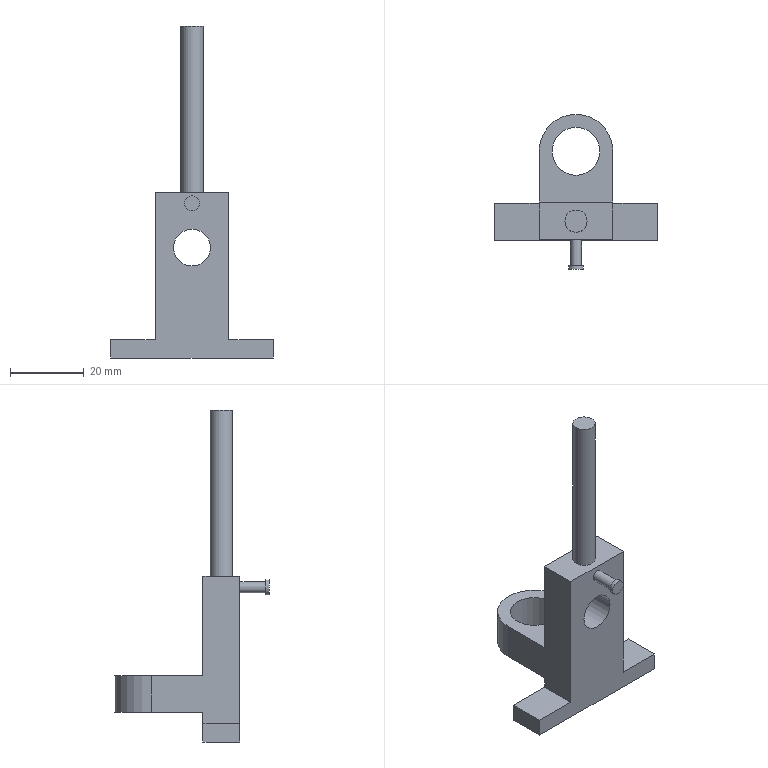Part | NX | features DATUM_CSYS 6, EXTRUDE 5, SKETCH 5 | 1 solid | 22 faces | box 44 x 42 x 89.9 mm | volume 13748 mm3 | plane 16 | cylinder 6 | commonest cylinder face diameters 3 x1 4 x1 6 x1 10 x1 13 x1 20 x1
STEP:
#1=CARTESIAN_POINT('',(-10.,5.,8.));
#2=VERTEX_POINT('',#1);
#3=CARTESIAN_POINT('',(-10.,5.,4.9));
#4=VERTEX_POINT('',#3);
#5=CARTESIAN_POINT('',(-10.,5.,44.9));
#6=DIRECTION('',(0.,0.,-1.));
#7=VECTOR('',#6,1000.);
#8=LINE('',#5,#7);
#9=EDGE_CURVE('',#2,#4,#8,.T.);
#10=ORIENTED_EDGE('',*,*,#9,.F.);
#11=CARTESIAN_POINT('',(10.,5.,8.));
#12=VERTEX_POINT('',#11);
#13=CARTESIAN_POINT('',(-10.,5.,8.));
#14=DIRECTION('',(1.,0.,0.));
#15=VECTOR('',#14,1000.);
#16=LINE('',#13,#15);
#17=EDGE_CURVE('',#2,#12,#16,.T.);
#18=ORIENTED_EDGE('',*,*,#17,.T.);
#19=CARTESIAN_POINT('',(10.,5.,4.9));
#20=VERTEX_POINT('',#19);
#21=CARTESIAN_POINT('',(10.,5.,4.9));
#22=DIRECTION('',(0.,0.,1.));
#23=VECTOR('',#22,1000.);
#24=LINE('',#21,#23);
#25=EDGE_CURVE('',#20,#12,#24,.T.);
#26=ORIENTED_EDGE('',*,*,#25,.F.);
#27=CARTESIAN_POINT('',(22.,5.,4.9));
#28=VERTEX_POINT('',#27);
#29=CARTESIAN_POINT('',(22.,5.,4.9));
#30=DIRECTION('',(-1.,0.,0.));
#31=VECTOR('',#30,1000.);
#32=LINE('',#29,#31);
#33=EDGE_CURVE('',#28,#20,#32,.T.);
#34=ORIENTED_EDGE('',*,*,#33,.F.);
#35=CARTESIAN_POINT('',(22.,5.,0.));
#36=VERTEX_POINT('',#35);
#37=CARTESIAN_POINT('',(22.,5.,0.));
#38=DIRECTION('',(0.,0.,1.));
#39=VECTOR('',#38,1000.);
#40=LINE('',#37,#39);
#41=EDGE_CURVE('',#36,#28,#40,.T.);
#42=ORIENTED_EDGE('',*,*,#41,.F.);
#43=CARTESIAN_POINT('',(-22.,5.,0.));
#44=VERTEX_POINT('',#43);
#45=CARTESIAN_POINT('',(0.,5.,0.));
#46=DIRECTION('',(1.,0.,0.));
#47=VECTOR('',#46,1000.);
#48=LINE('',#45,#47);
#49=EDGE_CURVE('',#44,#36,#48,.T.);
#50=ORIENTED_EDGE('',*,*,#49,.F.);
#51=CARTESIAN_POINT('',(-22.,5.,4.9));
#52=VERTEX_POINT('',#51);
#53=CARTESIAN_POINT('',(-22.,5.,4.9));
#54=DIRECTION('',(0.,0.,-1.));
#55=VECTOR('',#54,1000.);
#56=LINE('',#53,#55);
#57=EDGE_CURVE('',#52,#44,#56,.T.);
#58=ORIENTED_EDGE('',*,*,#57,.F.);
#59=CARTESIAN_POINT('',(-10.,5.,4.9));
#60=DIRECTION('',(-1.,0.,0.));
#61=VECTOR('',#60,1000.);
#62=LINE('',#59,#61);
#63=EDGE_CURVE('',#4,#52,#62,.T.);
#64=ORIENTED_EDGE('',*,*,#63,.F.);
#65=EDGE_LOOP('',(#10,#18,#26,#34,#42,#50,#58,#64));
#66=FACE_BOUND('',#65,.T.);
#67=CARTESIAN_POINT('',(0.,5.,29.9));
#68=DIRECTION('',(0.,1.,0.));
#69=DIRECTION('',(0.,0.,1.));
#70=AXIS2_PLACEMENT_3D('',#67,#68,#69);
#71=PLANE('',#70);
#72=ADVANCED_FACE('',(#66),#71,.T.);
#73=ORIENTED_EDGE('',*,*,#57,.T.);
#74=CARTESIAN_POINT('',(-22.,-5.,0.));
#75=VERTEX_POINT('',#74);
#76=CARTESIAN_POINT('',(-22.,-5.,0.));
#77=DIRECTION('',(0.,1.,0.));
#78=VECTOR('',#77,1000.);
#79=LINE('',#76,#78);
#80=EDGE_CURVE('',#75,#44,#79,.T.);
#81=ORIENTED_EDGE('',*,*,#80,.F.);
#82=CARTESIAN_POINT('',(-22.,-5.,4.9));
#83=VERTEX_POINT('',#82);
#84=CARTESIAN_POINT('',(-22.,-5.,4.9));
#85=DIRECTION('',(0.,0.,-1.));
#86=VECTOR('',#85,1000.);
#87=LINE('',#84,#86);
#88=EDGE_CURVE('',#83,#75,#87,.T.);
#89=ORIENTED_EDGE('',*,*,#88,.F.);
#90=CARTESIAN_POINT('',(-22.,-5.,4.9));
#91=DIRECTION('',(0.,1.,0.));
#92=VECTOR('',#91,1000.);
#93=LINE('',#90,#92);
#94=EDGE_CURVE('',#83,#52,#93,.T.);
#95=ORIENTED_EDGE('',*,*,#94,.T.);
#96=EDGE_LOOP('',(#73,#81,#89,#95));
#97=FACE_BOUND('',#96,.T.);
#98=CARTESIAN_POINT('',(-22.,-5.,4.9));
#99=DIRECTION('',(1.,0.,0.));
#100=DIRECTION('',(0.,0.,-1.));
#101=AXIS2_PLACEMENT_3D('',#98,#99,#100);
#102=PLANE('',#101);
#103=ADVANCED_FACE('',(#97),#102,.F.);
#104=ORIENTED_EDGE('',*,*,#49,.T.);
#105=CARTESIAN_POINT('',(22.,-5.,0.));
#106=VERTEX_POINT('',#105);
#107=CARTESIAN_POINT('',(22.,-5.,0.));
#108=DIRECTION('',(0.,1.,0.));
#109=VECTOR('',#108,1000.);
#110=LINE('',#107,#109);
#111=EDGE_CURVE('',#106,#36,#110,.T.);
#112=ORIENTED_EDGE('',*,*,#111,.F.);
#113=CARTESIAN_POINT('',(-22.,-5.,0.));
#114=DIRECTION('',(1.,0.,0.));
#115=VECTOR('',#114,1000.);
#116=LINE('',#113,#115);
#117=EDGE_CURVE('',#75,#106,#116,.T.);
#118=ORIENTED_EDGE('',*,*,#117,.F.);
#119=ORIENTED_EDGE('',*,*,#80,.T.);
#120=EDGE_LOOP('',(#104,#112,#118,#119));
#121=FACE_BOUND('',#120,.T.);
#122=CARTESIAN_POINT('',(0.,-5.,0.));
#123=DIRECTION('',(0.,0.,1.));
#124=DIRECTION('',(1.,0.,0.));
#125=AXIS2_PLACEMENT_3D('',#122,#123,#124);
#126=PLANE('',#125);
#127=ADVANCED_FACE('',(#121),#126,.F.);
#128=ORIENTED_EDGE('',*,*,#41,.T.);
#129=CARTESIAN_POINT('',(22.,-5.,4.9));
#130=VERTEX_POINT('',#129);
#131=CARTESIAN_POINT('',(22.,-5.,4.9));
#132=DIRECTION('',(0.,1.,0.));
#133=VECTOR('',#132,1000.);
#134=LINE('',#131,#133);
#135=EDGE_CURVE('',#130,#28,#134,.T.);
#136=ORIENTED_EDGE('',*,*,#135,.F.);
#137=CARTESIAN_POINT('',(22.,-5.,0.));
#138=DIRECTION('',(0.,0.,1.));
#139=VECTOR('',#138,1000.);
#140=LINE('',#137,#139);
#141=EDGE_CURVE('',#106,#130,#140,.T.);
#142=ORIENTED_EDGE('',*,*,#141,.F.);
#143=ORIENTED_EDGE('',*,*,#111,.T.);
#144=EDGE_LOOP('',(#128,#136,#142,#143));
#145=FACE_BOUND('',#144,.T.);
#146=CARTESIAN_POINT('',(22.,-5.,0.));
#147=DIRECTION('',(-1.,0.,0.));
#148=DIRECTION('',(0.,0.,1.));
#149=AXIS2_PLACEMENT_3D('',#146,#147,#148);
#150=PLANE('',#149);
#151=ADVANCED_FACE('',(#145),#150,.F.);
#152=ORIENTED_EDGE('',*,*,#33,.T.);
#153=CARTESIAN_POINT('',(10.,-5.,4.9));
#154=VERTEX_POINT('',#153);
#155=CARTESIAN_POINT('',(10.,-5.,4.9));
#156=DIRECTION('',(0.,1.,0.));
#157=VECTOR('',#156,1000.);
#158=LINE('',#155,#157);
#159=EDGE_CURVE('',#154,#20,#158,.T.);
#160=ORIENTED_EDGE('',*,*,#159,.F.);
#161=CARTESIAN_POINT('',(22.,-5.,4.9));
#162=DIRECTION('',(-1.,0.,0.));
#163=VECTOR('',#162,1000.);
#164=LINE('',#161,#163);
#165=EDGE_CURVE('',#130,#154,#164,.T.);
#166=ORIENTED_EDGE('',*,*,#165,.F.);
#167=ORIENTED_EDGE('',*,*,#135,.T.);
#168=EDGE_LOOP('',(#152,#160,#166,#167));
#169=FACE_BOUND('',#168,.T.);
#170=CARTESIAN_POINT('',(22.,-5.,4.9));
#171=DIRECTION('',(0.,0.,-1.));
#172=DIRECTION('',(-1.,0.,0.));
#173=AXIS2_PLACEMENT_3D('',#170,#171,#172);
#174=PLANE('',#173);
#175=ADVANCED_FACE('',(#169),#174,.F.);
#176=ORIENTED_EDGE('',*,*,#25,.T.);
#177=CARTESIAN_POINT('',(10.,19.,8.));
#178=VERTEX_POINT('',#177);
#179=CARTESIAN_POINT('',(10.,5.,8.));
#180=DIRECTION('',(0.,1.,0.));
#181=VECTOR('',#180,1000.);
#182=LINE('',#179,#181);
#183=EDGE_CURVE('',#12,#178,#182,.T.);
#184=ORIENTED_EDGE('',*,*,#183,.T.);
#185=CARTESIAN_POINT('',(10.,19.,18.));
#186=VERTEX_POINT('',#185);
#187=CARTESIAN_POINT('',(10.,19.,18.));
#188=DIRECTION('',(0.,0.,-1.));
#189=VECTOR('',#188,1000.);
#190=LINE('',#187,#189);
#191=EDGE_CURVE('',#186,#178,#190,.T.);
#192=ORIENTED_EDGE('',*,*,#191,.F.);
#193=CARTESIAN_POINT('',(10.,5.,18.));
#194=VERTEX_POINT('',#193);
#195=CARTESIAN_POINT('',(10.,5.,18.));
#196=DIRECTION('',(0.,1.,0.));
#197=VECTOR('',#196,1000.);
#198=LINE('',#195,#197);
#199=EDGE_CURVE('',#194,#186,#198,.T.);
#200=ORIENTED_EDGE('',*,*,#199,.F.);
#201=CARTESIAN_POINT('',(10.,5.,44.9));
#202=VERTEX_POINT('',#201);
#203=CARTESIAN_POINT('',(10.,5.,4.9));
#204=DIRECTION('',(0.,0.,1.));
#205=VECTOR('',#204,1000.);
#206=LINE('',#203,#205);
#207=EDGE_CURVE('',#194,#202,#206,.T.);
#208=ORIENTED_EDGE('',*,*,#207,.T.);
#209=CARTESIAN_POINT('',(10.,-5.,44.9));
#210=VERTEX_POINT('',#209);
#211=CARTESIAN_POINT('',(10.,-5.,44.9));
#212=DIRECTION('',(0.,1.,0.));
#213=VECTOR('',#212,1000.);
#214=LINE('',#211,#213);
#215=EDGE_CURVE('',#210,#202,#214,.T.);
#216=ORIENTED_EDGE('',*,*,#215,.F.);
#217=CARTESIAN_POINT('',(10.,-5.,4.9));
#218=DIRECTION('',(0.,0.,1.));
#219=VECTOR('',#218,1000.);
#220=LINE('',#217,#219);
#221=EDGE_CURVE('',#154,#210,#220,.T.);
#222=ORIENTED_EDGE('',*,*,#221,.F.);
#223=ORIENTED_EDGE('',*,*,#159,.T.);
#224=EDGE_LOOP('',(#176,#184,#192,#200,#208,#216,#222,#223));
#225=FACE_BOUND('',#224,.T.);
#226=CARTESIAN_POINT('',(10.,-5.,4.9));
#227=DIRECTION('',(-1.,0.,0.));
#228=DIRECTION('',(0.,0.,1.));
#229=AXIS2_PLACEMENT_3D('',#226,#227,#228);
#230=PLANE('',#229);
#231=ADVANCED_FACE('',(#225),#230,.F.);
#232=CARTESIAN_POINT('',(-3.,0.,44.9));
#233=VERTEX_POINT('',#232);
#234=CARTESIAN_POINT('',(0.,0.,44.9));
#235=DIRECTION('',(0.,0.,-1.));
#236=DIRECTION('',(-1.,0.,0.));
#237=AXIS2_PLACEMENT_3D('',#234,#235,#236);
#238=CIRCLE('',#237,3.);
#239=EDGE_CURVE('',#233,#233,#238,.T.);
#240=ORIENTED_EDGE('',*,*,#239,.T.);
#241=EDGE_LOOP('',(#240));
#242=FACE_BOUND('',#241,.T.);
#243=CARTESIAN_POINT('',(-10.,5.,44.9));
#244=VERTEX_POINT('',#243);
#245=CARTESIAN_POINT('',(0.,5.,44.9));
#246=DIRECTION('',(-1.,0.,0.));
#247=VECTOR('',#246,1000.);
#248=LINE('',#245,#247);
#249=EDGE_CURVE('',#202,#244,#248,.T.);
#250=ORIENTED_EDGE('',*,*,#249,.T.);
#251=CARTESIAN_POINT('',(-10.,-5.,44.9));
#252=VERTEX_POINT('',#251);
#253=CARTESIAN_POINT('',(-10.,-5.,44.9));
#254=DIRECTION('',(0.,1.,0.));
#255=VECTOR('',#254,1000.);
#256=LINE('',#253,#255);
#257=EDGE_CURVE('',#252,#244,#256,.T.);
#258=ORIENTED_EDGE('',*,*,#257,.F.);
#259=CARTESIAN_POINT('',(10.,-5.,44.9));
#260=DIRECTION('',(-1.,0.,0.));
#261=VECTOR('',#260,1000.);
#262=LINE('',#259,#261);
#263=EDGE_CURVE('',#210,#252,#262,.T.);
#264=ORIENTED_EDGE('',*,*,#263,.F.);
#265=ORIENTED_EDGE('',*,*,#215,.T.);
#266=EDGE_LOOP('',(#250,#258,#264,#265));
#267=FACE_BOUND('',#266,.T.);
#268=CARTESIAN_POINT('',(0.,-5.,44.9));
#269=DIRECTION('',(0.,0.,-1.));
#270=DIRECTION('',(-1.,0.,0.));
#271=AXIS2_PLACEMENT_3D('',#268,#269,#270);
#272=PLANE('',#271);
#273=ADVANCED_FACE('',(#242,#267),#272,.F.);
#274=CARTESIAN_POINT('',(-10.,5.,18.));
#275=VERTEX_POINT('',#274);
#276=CARTESIAN_POINT('',(-10.,5.,44.9));
#277=DIRECTION('',(0.,0.,-1.));
#278=VECTOR('',#277,1000.);
#279=LINE('',#276,#278);
#280=EDGE_CURVE('',#244,#275,#279,.T.);
#281=ORIENTED_EDGE('',*,*,#280,.T.);
#282=CARTESIAN_POINT('',(-10.,19.,18.));
#283=VERTEX_POINT('',#282);
#284=CARTESIAN_POINT('',(-10.,19.,18.));
#285=DIRECTION('',(0.,-1.,0.));
#286=VECTOR('',#285,1000.);
#287=LINE('',#284,#286);
#288=EDGE_CURVE('',#283,#275,#287,.T.);
#289=ORIENTED_EDGE('',*,*,#288,.F.);
#290=CARTESIAN_POINT('',(-10.,19.,8.));
#291=VERTEX_POINT('',#290);
#292=CARTESIAN_POINT('',(-10.,19.,18.));
#293=DIRECTION('',(0.,0.,-1.));
#294=VECTOR('',#293,1000.);
#295=LINE('',#292,#294);
#296=EDGE_CURVE('',#283,#291,#295,.T.);
#297=ORIENTED_EDGE('',*,*,#296,.T.);
#298=CARTESIAN_POINT('',(-10.,19.,8.));
#299=DIRECTION('',(0.,-1.,0.));
#300=VECTOR('',#299,1000.);
#301=LINE('',#298,#300);
#302=EDGE_CURVE('',#291,#2,#301,.T.);
#303=ORIENTED_EDGE('',*,*,#302,.T.);
#304=ORIENTED_EDGE('',*,*,#9,.T.);
#305=CARTESIAN_POINT('',(-10.,-5.,4.9));
#306=VERTEX_POINT('',#305);
#307=CARTESIAN_POINT('',(-10.,-5.,4.9));
#308=DIRECTION('',(0.,1.,0.));
#309=VECTOR('',#308,1000.);
#310=LINE('',#307,#309);
#311=EDGE_CURVE('',#306,#4,#310,.T.);
#312=ORIENTED_EDGE('',*,*,#311,.F.);
#313=CARTESIAN_POINT('',(-10.,-5.,44.9));
#314=DIRECTION('',(0.,0.,-1.));
#315=VECTOR('',#314,1000.);
#316=LINE('',#313,#315);
#317=EDGE_CURVE('',#252,#306,#316,.T.);
#318=ORIENTED_EDGE('',*,*,#317,.F.);
#319=ORIENTED_EDGE('',*,*,#257,.T.);
#320=EDGE_LOOP('',(#281,#289,#297,#303,#304,#312,#318,#319));
#321=FACE_BOUND('',#320,.T.);
#322=CARTESIAN_POINT('',(-10.,-5.,44.9));
#323=DIRECTION('',(1.,0.,0.));
#324=DIRECTION('',(0.,0.,-1.));
#325=AXIS2_PLACEMENT_3D('',#322,#323,#324);
#326=PLANE('',#325);
#327=ADVANCED_FACE('',(#321),#326,.F.);
#328=ORIENTED_EDGE('',*,*,#63,.T.);
#329=ORIENTED_EDGE('',*,*,#94,.F.);
#330=CARTESIAN_POINT('',(-10.,-5.,4.9));
#331=DIRECTION('',(-1.,0.,0.));
#332=VECTOR('',#331,1000.);
#333=LINE('',#330,#332);
#334=EDGE_CURVE('',#306,#83,#333,.T.);
#335=ORIENTED_EDGE('',*,*,#334,.F.);
#336=ORIENTED_EDGE('',*,*,#311,.T.);
#337=EDGE_LOOP('',(#328,#329,#335,#336));
#338=FACE_BOUND('',#337,.T.);
#339=CARTESIAN_POINT('',(-10.,-5.,4.9));
#340=DIRECTION('',(0.,0.,-1.));
#341=DIRECTION('',(-1.,0.,0.));
#342=AXIS2_PLACEMENT_3D('',#339,#340,#341);
#343=PLANE('',#342);
#344=ADVANCED_FACE('',(#338),#343,.F.);
#345=CARTESIAN_POINT('',(5.,-5.,29.9));
#346=VERTEX_POINT('',#345);
#347=CARTESIAN_POINT('',(0.,-5.,29.9));
#348=DIRECTION('',(0.,1.,0.));
#349=DIRECTION('',(1.,0.,0.));
#350=AXIS2_PLACEMENT_3D('',#347,#348,#349);
#351=CIRCLE('',#350,5.);
#352=EDGE_CURVE('',#346,#346,#351,.T.);
#353=ORIENTED_EDGE('',*,*,#352,.F.);
#354=EDGE_LOOP('',(#353));
#355=FACE_BOUND('',#354,.T.);
#356=CARTESIAN_POINT('',(5.,5.,29.9));
#357=VERTEX_POINT('',#356);
#358=CARTESIAN_POINT('',(0.,5.,29.9));
#359=DIRECTION('',(0.,1.,0.));
#360=DIRECTION('',(1.,0.,0.));
#361=AXIS2_PLACEMENT_3D('',#358,#359,#360);
#362=CIRCLE('',#361,5.);
#363=EDGE_CURVE('',#357,#357,#362,.T.);
#364=ORIENTED_EDGE('',*,*,#363,.T.);
#365=EDGE_LOOP('',(#364));
#366=FACE_BOUND('',#365,.T.);
#367=CARTESIAN_POINT('',(0.,-5.,29.9));
#368=DIRECTION('',(0.,1.,0.));
#369=DIRECTION('',(0.,0.,1.));
#370=AXIS2_PLACEMENT_3D('',#367,#368,#369);
#371=CYLINDRICAL_SURFACE('',#370,5.);
#372=ADVANCED_FACE('',(#355,#366),#371,.F.);
#373=CARTESIAN_POINT('',(1.5,-5.,41.9));
#374=VERTEX_POINT('',#373);
#375=CARTESIAN_POINT('',(0.,-5.,41.9));
#376=DIRECTION('',(0.,1.,0.));
#377=DIRECTION('',(1.,0.,0.));
#378=AXIS2_PLACEMENT_3D('',#375,#376,#377);
#379=CIRCLE('',#378,1.5);
#380=EDGE_CURVE('',#374,#374,#379,.T.);
#381=ORIENTED_EDGE('',*,*,#380,.T.);
#382=EDGE_LOOP('',(#381));
#383=FACE_BOUND('',#382,.T.);
#384=ORIENTED_EDGE('',*,*,#88,.T.);
#385=ORIENTED_EDGE('',*,*,#117,.T.);
#386=ORIENTED_EDGE('',*,*,#141,.T.);
#387=ORIENTED_EDGE('',*,*,#165,.T.);
#388=ORIENTED_EDGE('',*,*,#221,.T.);
#389=ORIENTED_EDGE('',*,*,#263,.T.);
#390=ORIENTED_EDGE('',*,*,#317,.T.);
#391=ORIENTED_EDGE('',*,*,#334,.T.);
#392=EDGE_LOOP('',(#384,#385,#386,#387,#388,#389,#390,#391));
#393=FACE_BOUND('',#392,.T.);
#394=ORIENTED_EDGE('',*,*,#352,.T.);
#395=EDGE_LOOP('',(#394));
#396=FACE_BOUND('',#395,.T.);
#397=CARTESIAN_POINT('',(0.,-5.,29.9));
#398=DIRECTION('',(0.,1.,0.));
#399=DIRECTION('',(0.,0.,1.));
#400=AXIS2_PLACEMENT_3D('',#397,#398,#399);
#401=PLANE('',#400);
#402=ADVANCED_FACE('',(#383,#393,#396),#401,.F.);
#403=CARTESIAN_POINT('',(-10.,5.,18.));
#404=DIRECTION('',(1.,0.,0.));
#405=VECTOR('',#404,1000.);
#406=LINE('',#403,#405);
#407=EDGE_CURVE('',#275,#194,#406,.T.);
#408=ORIENTED_EDGE('',*,*,#407,.F.);
#409=ORIENTED_EDGE('',*,*,#280,.F.);
#410=ORIENTED_EDGE('',*,*,#249,.F.);
#411=ORIENTED_EDGE('',*,*,#207,.F.);
#412=EDGE_LOOP('',(#408,#409,#410,#411));
#413=FACE_BOUND('',#412,.T.);
#414=ORIENTED_EDGE('',*,*,#363,.F.);
#415=EDGE_LOOP('',(#414));
#416=FACE_BOUND('',#415,.T.);
#417=CARTESIAN_POINT('',(0.,5.,29.9));
#418=DIRECTION('',(0.,1.,0.));
#419=DIRECTION('',(0.,0.,1.));
#420=AXIS2_PLACEMENT_3D('',#417,#418,#419);
#421=PLANE('',#420);
#422=ADVANCED_FACE('',(#413,#416),#421,.T.);
#423=CARTESIAN_POINT('',(3.,0.,89.9));
#424=VERTEX_POINT('',#423);
#425=CARTESIAN_POINT('',(0.,0.,89.9));
#426=DIRECTION('',(0.,0.,1.));
#427=DIRECTION('',(1.,0.,0.));
#428=AXIS2_PLACEMENT_3D('',#425,#426,#427);
#429=CIRCLE('',#428,3.);
#430=EDGE_CURVE('',#424,#424,#429,.T.);
#431=ORIENTED_EDGE('',*,*,#430,.F.);
#432=EDGE_LOOP('',(#431));
#433=FACE_BOUND('',#432,.T.);
#434=ORIENTED_EDGE('',*,*,#239,.F.);
#435=EDGE_LOOP('',(#434));
#436=FACE_BOUND('',#435,.T.);
#437=CARTESIAN_POINT('',(0.,0.,89.9));
#438=DIRECTION('',(0.,0.,-1.));
#439=DIRECTION('',(-1.,0.,0.));
#440=AXIS2_PLACEMENT_3D('',#437,#438,#439);
#441=CYLINDRICAL_SURFACE('',#440,3.);
#442=ADVANCED_FACE('',(#433,#436),#441,.T.);
#443=ORIENTED_EDGE('',*,*,#430,.T.);
#444=EDGE_LOOP('',(#443));
#445=FACE_BOUND('',#444,.T.);
#446=CARTESIAN_POINT('',(0.,0.,89.9));
#447=DIRECTION('',(0.,0.,1.));
#448=DIRECTION('',(1.,0.,0.));
#449=AXIS2_PLACEMENT_3D('',#446,#447,#448);
#450=PLANE('',#449);
#451=ADVANCED_FACE('',(#445),#450,.T.);
#452=CARTESIAN_POINT('',(1.5,-12.,41.9));
#453=VERTEX_POINT('',#452);
#454=CARTESIAN_POINT('',(0.,-12.,41.9));
#455=DIRECTION('',(0.,1.,0.));
#456=DIRECTION('',(1.,0.,0.));
#457=AXIS2_PLACEMENT_3D('',#454,#455,#456);
#458=CIRCLE('',#457,1.5);
#459=EDGE_CURVE('',#453,#453,#458,.T.);
#460=ORIENTED_EDGE('',*,*,#459,.T.);
#461=EDGE_LOOP('',(#460));
#462=FACE_BOUND('',#461,.T.);
#463=ORIENTED_EDGE('',*,*,#380,.F.);
#464=EDGE_LOOP('',(#463));
#465=FACE_BOUND('',#464,.T.);
#466=CARTESIAN_POINT('',(0.,-12.,41.9));
#467=DIRECTION('',(0.,1.,0.));
#468=DIRECTION('',(0.,0.,1.));
#469=AXIS2_PLACEMENT_3D('',#466,#467,#468);
#470=CYLINDRICAL_SURFACE('',#469,1.5);
#471=ADVANCED_FACE('',(#462,#465),#470,.T.);
#472=CARTESIAN_POINT('',(-2.,-13.,41.9));
#473=VERTEX_POINT('',#472);
#474=CARTESIAN_POINT('',(0.,-13.,41.9));
#475=DIRECTION('',(0.,1.,0.));
#476=DIRECTION('',(-1.,0.,0.));
#477=AXIS2_PLACEMENT_3D('',#474,#475,#476);
#478=CIRCLE('',#477,2.);
#479=EDGE_CURVE('',#473,#473,#478,.T.);
#480=ORIENTED_EDGE('',*,*,#479,.T.);
#481=EDGE_LOOP('',(#480));
#482=FACE_BOUND('',#481,.T.);
#483=CARTESIAN_POINT('',(-2.,-12.,41.9));
#484=VERTEX_POINT('',#483);
#485=CARTESIAN_POINT('',(0.,-12.,41.9));
#486=DIRECTION('',(0.,1.,0.));
#487=DIRECTION('',(-1.,0.,0.));
#488=AXIS2_PLACEMENT_3D('',#485,#486,#487);
#489=CIRCLE('',#488,2.);
#490=EDGE_CURVE('',#484,#484,#489,.T.);
#491=ORIENTED_EDGE('',*,*,#490,.F.);
#492=EDGE_LOOP('',(#491));
#493=FACE_BOUND('',#492,.T.);
#494=CARTESIAN_POINT('',(0.,-13.,41.9));
#495=DIRECTION('',(0.,1.,0.));
#496=DIRECTION('',(0.,0.,1.));
#497=AXIS2_PLACEMENT_3D('',#494,#495,#496);
#498=CYLINDRICAL_SURFACE('',#497,2.);
#499=ADVANCED_FACE('',(#482,#493),#498,.T.);
#500=ORIENTED_EDGE('',*,*,#479,.F.);
#501=EDGE_LOOP('',(#500));
#502=FACE_BOUND('',#501,.T.);
#503=CARTESIAN_POINT('',(0.,-13.,41.9));
#504=DIRECTION('',(0.,1.,0.));
#505=DIRECTION('',(0.,0.,1.));
#506=AXIS2_PLACEMENT_3D('',#503,#504,#505);
#507=PLANE('',#506);
#508=ADVANCED_FACE('',(#502),#507,.F.);
#509=ORIENTED_EDGE('',*,*,#459,.F.);
#510=EDGE_LOOP('',(#509));
#511=FACE_BOUND('',#510,.T.);
#512=ORIENTED_EDGE('',*,*,#490,.T.);
#513=EDGE_LOOP('',(#512));
#514=FACE_BOUND('',#513,.T.);
#515=CARTESIAN_POINT('',(0.,-12.,41.9));
#516=DIRECTION('',(0.,1.,0.));
#517=DIRECTION('',(0.,0.,1.));
#518=AXIS2_PLACEMENT_3D('',#515,#516,#517);
#519=PLANE('',#518);
#520=ADVANCED_FACE('',(#511,#514),#519,.T.);
#521=CARTESIAN_POINT('',(0.,19.,8.));
#522=DIRECTION('',(0.,0.,1.));
#523=DIRECTION('',(0.,-1.,0.));
#524=AXIS2_PLACEMENT_3D('',#521,#522,#523);
#525=CIRCLE('',#524,10.);
#526=EDGE_CURVE('',#178,#291,#525,.T.);
#527=ORIENTED_EDGE('',*,*,#526,.T.);
#528=ORIENTED_EDGE('',*,*,#296,.F.);
#529=CARTESIAN_POINT('',(0.,19.,18.));
#530=DIRECTION('',(0.,0.,1.));
#531=DIRECTION('',(0.,-1.,0.));
#532=AXIS2_PLACEMENT_3D('',#529,#530,#531);
#533=CIRCLE('',#532,10.);
#534=EDGE_CURVE('',#186,#283,#533,.T.);
#535=ORIENTED_EDGE('',*,*,#534,.F.);
#536=ORIENTED_EDGE('',*,*,#191,.T.);
#537=EDGE_LOOP('',(#527,#528,#535,#536));
#538=FACE_BOUND('',#537,.T.);
#539=CARTESIAN_POINT('',(0.,19.,18.));
#540=DIRECTION('',(0.,0.,-1.));
#541=DIRECTION('',(-1.,0.,0.));
#542=AXIS2_PLACEMENT_3D('',#539,#540,#541);
#543=CYLINDRICAL_SURFACE('',#542,10.);
#544=ADVANCED_FACE('',(#538),#543,.T.);
#545=CARTESIAN_POINT('',(0.,25.5,18.));
#546=VERTEX_POINT('',#545);
#547=CARTESIAN_POINT('',(0.,19.,18.));
#548=DIRECTION('',(0.,0.,1.));
#549=DIRECTION('',(0.,1.,0.));
#550=AXIS2_PLACEMENT_3D('',#547,#548,#549);
#551=CIRCLE('',#550,6.5);
#552=EDGE_CURVE('',#546,#546,#551,.T.);
#553=ORIENTED_EDGE('',*,*,#552,.T.);
#554=EDGE_LOOP('',(#553));
#555=FACE_BOUND('',#554,.T.);
#556=CARTESIAN_POINT('',(0.,25.5,8.));
#557=VERTEX_POINT('',#556);
#558=CARTESIAN_POINT('',(0.,19.,8.));
#559=DIRECTION('',(0.,0.,1.));
#560=DIRECTION('',(0.,1.,0.));
#561=AXIS2_PLACEMENT_3D('',#558,#559,#560);
#562=CIRCLE('',#561,6.5);
#563=EDGE_CURVE('',#557,#557,#562,.T.);
#564=ORIENTED_EDGE('',*,*,#563,.F.);
#565=EDGE_LOOP('',(#564));
#566=FACE_BOUND('',#565,.T.);
#567=CARTESIAN_POINT('',(0.,19.,18.));
#568=DIRECTION('',(0.,0.,-1.));
#569=DIRECTION('',(-1.,0.,0.));
#570=AXIS2_PLACEMENT_3D('',#567,#568,#569);
#571=CYLINDRICAL_SURFACE('',#570,6.5);
#572=ADVANCED_FACE('',(#555,#566),#571,.F.);
#573=ORIENTED_EDGE('',*,*,#288,.T.);
#574=ORIENTED_EDGE('',*,*,#407,.T.);
#575=ORIENTED_EDGE('',*,*,#199,.T.);
#576=ORIENTED_EDGE('',*,*,#534,.T.);
#577=EDGE_LOOP('',(#573,#574,#575,#576));
#578=FACE_BOUND('',#577,.T.);
#579=ORIENTED_EDGE('',*,*,#552,.F.);
#580=EDGE_LOOP('',(#579));
#581=FACE_BOUND('',#580,.T.);
#582=CARTESIAN_POINT('',(0.,19.,18.));
#583=DIRECTION('',(0.,0.,1.));
#584=DIRECTION('',(1.,0.,0.));
#585=AXIS2_PLACEMENT_3D('',#582,#583,#584);
#586=PLANE('',#585);
#587=ADVANCED_FACE('',(#578,#581),#586,.T.);
#588=ORIENTED_EDGE('',*,*,#302,.F.);
#589=ORIENTED_EDGE('',*,*,#526,.F.);
#590=ORIENTED_EDGE('',*,*,#183,.F.);
#591=ORIENTED_EDGE('',*,*,#17,.F.);
#592=EDGE_LOOP('',(#588,#589,#590,#591));
#593=FACE_BOUND('',#592,.T.);
#594=ORIENTED_EDGE('',*,*,#563,.T.);
#595=EDGE_LOOP('',(#594));
#596=FACE_BOUND('',#595,.T.);
#597=CARTESIAN_POINT('',(0.,19.,8.));
#598=DIRECTION('',(0.,0.,1.));
#599=DIRECTION('',(1.,0.,0.));
#600=AXIS2_PLACEMENT_3D('',#597,#598,#599);
#601=PLANE('',#600);
#602=ADVANCED_FACE('',(#593,#596),#601,.F.);
#603=CLOSED_SHELL('',(#72,#103,#127,#151,#175,#231,#273,#327,#344,#372,#402,#422,#442,#451,#471,#499,#508,#520,#544,#572,#587,#602));
#604=MANIFOLD_SOLID_BREP('',#603);
#605=(LENGTH_UNIT()NAMED_UNIT(*)SI_UNIT(.MILLI.,.METRE.));
#606=UNCERTAINTY_MEASURE_WITH_UNIT(LENGTH_MEASURE(0.00001),#605,'','');
#607=(NAMED_UNIT(*)PLANE_ANGLE_UNIT()SI_UNIT($,.RADIAN.));
#608=(NAMED_UNIT(*)SI_UNIT($,.STERADIAN.)SOLID_ANGLE_UNIT());
#609=(GEOMETRIC_REPRESENTATION_CONTEXT(3)GLOBAL_UNCERTAINTY_ASSIGNED_CONTEXT((#606))GLOBAL_UNIT_ASSIGNED_CONTEXT((#605,#607,#608))REPRESENTATION_CONTEXT('',''));
#610=ADVANCED_BREP_SHAPE_REPRESENTATION('',(#604),#609);